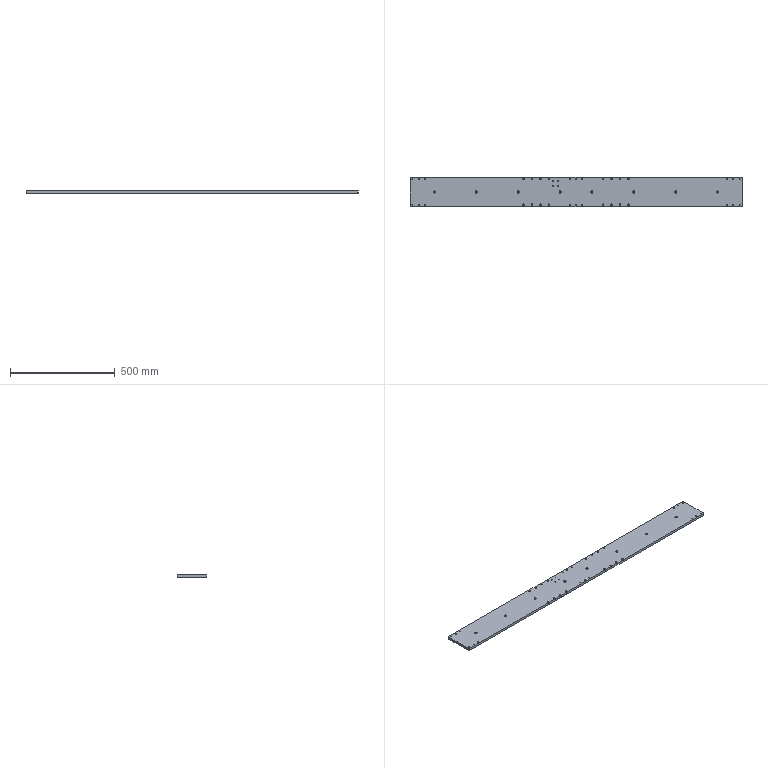Part | STEP file | 0-19-01 Sliding plate | 1 solid | 238 faces | box 1583 x 140 x 12 mm | volume 2630174 mm3 | cylinder 140 | plane 98 | commonest cylinder face diameters 6.6 x48 11 x48 5 x36 4.2 x8